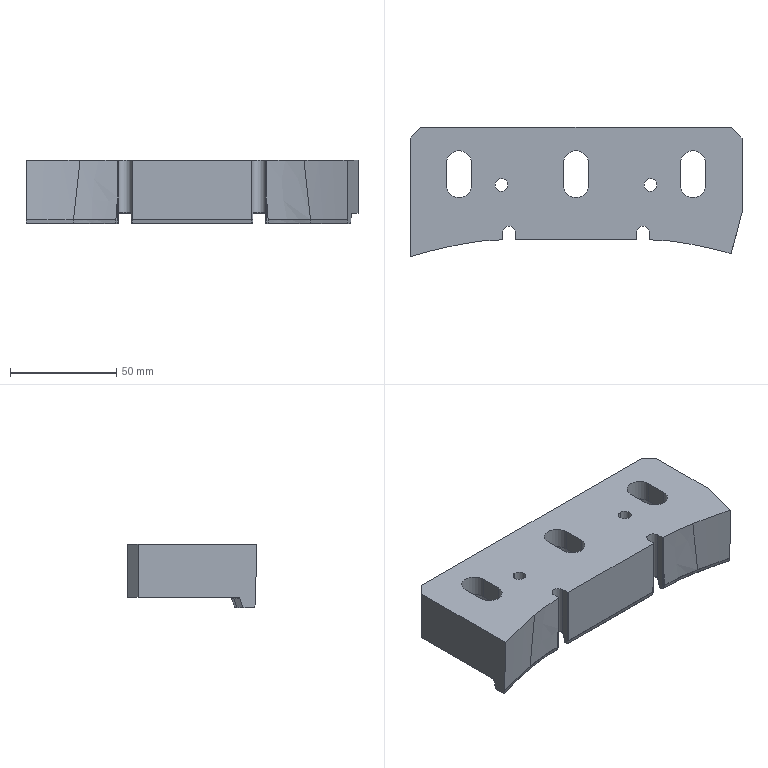Part | 1 solid | 214 faces | box 156 x 60.706 x 30 mm | volume 170936 mm3 | plane 84 | cylinder 50 | other 26 | spline 22 | torus 14 | sphere 12 | cone 6 | commonest cylinder face diameters 1 x28 6 x6 12 x6 24 x6 8 x4